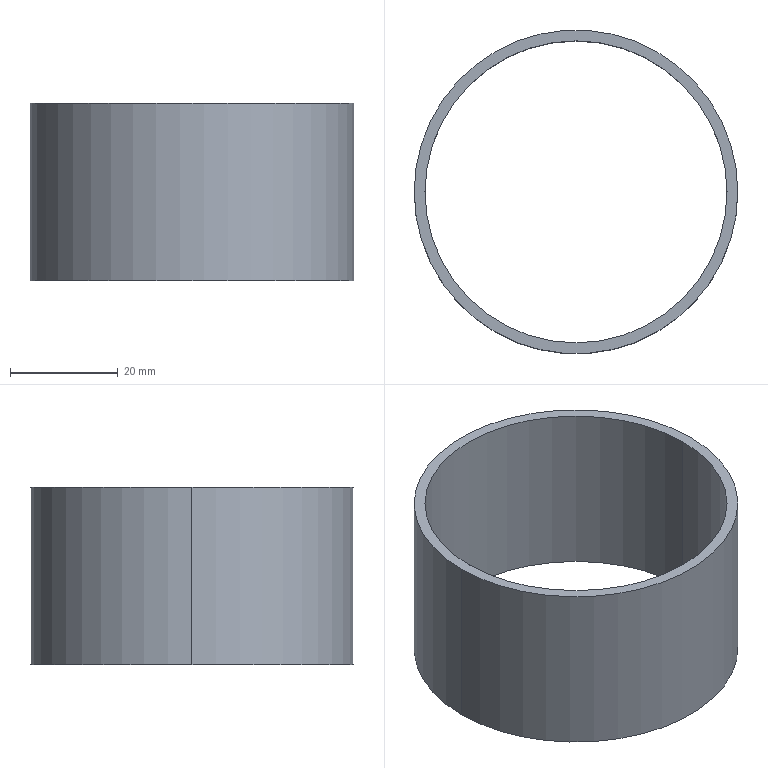Part | SolidWorks | features Extrusion 1 | 1 solid | 6 faces | box 60 x 60 x 33 mm | volume 12026 mm3 | cylinder 4 | plane 2 | commonest cylinder face diameters 56 x2 60 x2
STEP:
#1=CARTESIAN_POINT('',(-28.,0.,33.));
#2=VERTEX_POINT('',#1);
#3=CARTESIAN_POINT('',(28.,0.,33.));
#4=VERTEX_POINT('',#3);
#5=CARTESIAN_POINT('',(0.,0.,33.));
#6=DIRECTION('',(0.,0.,1.));
#7=DIRECTION('',(1.,0.,0.));
#8=AXIS2_PLACEMENT_3D('',#5,#6,#7);
#9=CIRCLE('',#8,28.);
#10=EDGE_CURVE('',#2,#4,#9,.T.);
#11=ORIENTED_EDGE('',*,*,#10,.T.);
#12=CARTESIAN_POINT('',(28.,0.,0.));
#13=VERTEX_POINT('',#12);
#14=CARTESIAN_POINT('',(28.,0.,33.));
#15=DIRECTION('',(0.,0.,-1.));
#16=VECTOR('',#15,1000.);
#17=LINE('',#14,#16);
#18=EDGE_CURVE('',#4,#13,#17,.T.);
#19=ORIENTED_EDGE('',*,*,#18,.T.);
#20=CARTESIAN_POINT('',(-28.,0.,0.));
#21=VERTEX_POINT('',#20);
#22=CARTESIAN_POINT('',(0.,0.,0.));
#23=DIRECTION('',(0.,0.,1.));
#24=DIRECTION('',(1.,0.,0.));
#25=AXIS2_PLACEMENT_3D('',#22,#23,#24);
#26=CIRCLE('',#25,28.);
#27=EDGE_CURVE('',#21,#13,#26,.T.);
#28=ORIENTED_EDGE('',*,*,#27,.F.);
#29=CARTESIAN_POINT('',(-28.,0.,33.));
#30=DIRECTION('',(0.,0.,-1.));
#31=VECTOR('',#30,1000.);
#32=LINE('',#29,#31);
#33=EDGE_CURVE('',#2,#21,#32,.T.);
#34=ORIENTED_EDGE('',*,*,#33,.F.);
#35=EDGE_LOOP('',(#11,#19,#28,#34));
#36=FACE_OUTER_BOUND('',#35,.T.);
#37=CARTESIAN_POINT('',(0.,0.,33.));
#38=DIRECTION('',(0.,0.,-1.));
#39=DIRECTION('',(-1.,0.,0.));
#40=AXIS2_PLACEMENT_3D('',#37,#38,#39);
#41=CYLINDRICAL_SURFACE('',#40,28.);
#42=ADVANCED_FACE('',(#36),#41,.F.);
#43=CARTESIAN_POINT('',(30.,0.,33.));
#44=VERTEX_POINT('',#43);
#45=CARTESIAN_POINT('',(-30.,0.,33.));
#46=VERTEX_POINT('',#45);
#47=CARTESIAN_POINT('',(0.,0.,33.));
#48=DIRECTION('',(0.,0.,1.));
#49=DIRECTION('',(1.,0.,0.));
#50=AXIS2_PLACEMENT_3D('',#47,#48,#49);
#51=CIRCLE('',#50,30.);
#52=EDGE_CURVE('',#44,#46,#51,.T.);
#53=ORIENTED_EDGE('',*,*,#52,.F.);
#54=CARTESIAN_POINT('',(30.,0.,0.));
#55=VERTEX_POINT('',#54);
#56=CARTESIAN_POINT('',(30.,0.,33.));
#57=DIRECTION('',(0.,0.,-1.));
#58=VECTOR('',#57,1000.);
#59=LINE('',#56,#58);
#60=EDGE_CURVE('',#44,#55,#59,.T.);
#61=ORIENTED_EDGE('',*,*,#60,.T.);
#62=CARTESIAN_POINT('',(-30.,0.,0.));
#63=VERTEX_POINT('',#62);
#64=CARTESIAN_POINT('',(0.,0.,0.));
#65=DIRECTION('',(0.,0.,1.));
#66=DIRECTION('',(1.,0.,0.));
#67=AXIS2_PLACEMENT_3D('',#64,#65,#66);
#68=CIRCLE('',#67,30.);
#69=EDGE_CURVE('',#55,#63,#68,.T.);
#70=ORIENTED_EDGE('',*,*,#69,.T.);
#71=CARTESIAN_POINT('',(-30.,0.,33.));
#72=DIRECTION('',(0.,0.,-1.));
#73=VECTOR('',#72,1000.);
#74=LINE('',#71,#73);
#75=EDGE_CURVE('',#46,#63,#74,.T.);
#76=ORIENTED_EDGE('',*,*,#75,.F.);
#77=EDGE_LOOP('',(#53,#61,#70,#76));
#78=FACE_OUTER_BOUND('',#77,.T.);
#79=CARTESIAN_POINT('',(0.,0.,33.));
#80=DIRECTION('',(0.,0.,-1.));
#81=DIRECTION('',(-1.,0.,0.));
#82=AXIS2_PLACEMENT_3D('',#79,#80,#81);
#83=CYLINDRICAL_SURFACE('',#82,30.);
#84=ADVANCED_FACE('',(#78),#83,.T.);
#85=CARTESIAN_POINT('',(0.,0.,33.));
#86=DIRECTION('',(0.,0.,1.));
#87=DIRECTION('',(1.,0.,0.));
#88=AXIS2_PLACEMENT_3D('',#85,#86,#87);
#89=CIRCLE('',#88,30.);
#90=EDGE_CURVE('',#46,#44,#89,.T.);
#91=ORIENTED_EDGE('',*,*,#90,.T.);
#92=ORIENTED_EDGE('',*,*,#52,.T.);
#93=EDGE_LOOP('',(#91,#92));
#94=FACE_OUTER_BOUND('',#93,.T.);
#95=ORIENTED_EDGE('',*,*,#10,.F.);
#96=CARTESIAN_POINT('',(0.,0.,33.));
#97=DIRECTION('',(0.,0.,1.));
#98=DIRECTION('',(1.,0.,0.));
#99=AXIS2_PLACEMENT_3D('',#96,#97,#98);
#100=CIRCLE('',#99,28.);
#101=EDGE_CURVE('',#4,#2,#100,.T.);
#102=ORIENTED_EDGE('',*,*,#101,.F.);
#103=EDGE_LOOP('',(#95,#102));
#104=FACE_BOUND('',#103,.T.);
#105=CARTESIAN_POINT('',(0.,0.,33.));
#106=DIRECTION('',(0.,0.,1.));
#107=DIRECTION('',(1.,0.,0.));
#108=AXIS2_PLACEMENT_3D('',#105,#106,#107);
#109=PLANE('',#108);
#110=ADVANCED_FACE('',(#94,#104),#109,.T.);
#111=CARTESIAN_POINT('',(0.,0.,0.));
#112=DIRECTION('',(0.,0.,1.));
#113=DIRECTION('',(1.,0.,0.));
#114=AXIS2_PLACEMENT_3D('',#111,#112,#113);
#115=CIRCLE('',#114,30.);
#116=EDGE_CURVE('',#63,#55,#115,.T.);
#117=ORIENTED_EDGE('',*,*,#116,.F.);
#118=ORIENTED_EDGE('',*,*,#69,.F.);
#119=EDGE_LOOP('',(#117,#118));
#120=FACE_OUTER_BOUND('',#119,.T.);
#121=ORIENTED_EDGE('',*,*,#27,.T.);
#122=CARTESIAN_POINT('',(0.,0.,0.));
#123=DIRECTION('',(0.,0.,1.));
#124=DIRECTION('',(1.,0.,0.));
#125=AXIS2_PLACEMENT_3D('',#122,#123,#124);
#126=CIRCLE('',#125,28.);
#127=EDGE_CURVE('',#13,#21,#126,.T.);
#128=ORIENTED_EDGE('',*,*,#127,.T.);
#129=EDGE_LOOP('',(#121,#128));
#130=FACE_BOUND('',#129,.T.);
#131=CARTESIAN_POINT('',(0.,0.,0.));
#132=DIRECTION('',(0.,0.,1.));
#133=DIRECTION('',(1.,0.,0.));
#134=AXIS2_PLACEMENT_3D('',#131,#132,#133);
#135=PLANE('',#134);
#136=ADVANCED_FACE('',(#120,#130),#135,.F.);
#137=ORIENTED_EDGE('',*,*,#60,.F.);
#138=ORIENTED_EDGE('',*,*,#90,.F.);
#139=ORIENTED_EDGE('',*,*,#75,.T.);
#140=ORIENTED_EDGE('',*,*,#116,.T.);
#141=EDGE_LOOP('',(#137,#138,#139,#140));
#142=FACE_OUTER_BOUND('',#141,.T.);
#143=CARTESIAN_POINT('',(0.,0.,33.));
#144=DIRECTION('',(0.,0.,-1.));
#145=DIRECTION('',(-1.,0.,0.));
#146=AXIS2_PLACEMENT_3D('',#143,#144,#145);
#147=CYLINDRICAL_SURFACE('',#146,30.);
#148=ADVANCED_FACE('',(#142),#147,.T.);
#149=ORIENTED_EDGE('',*,*,#18,.F.);
#150=ORIENTED_EDGE('',*,*,#101,.T.);
#151=ORIENTED_EDGE('',*,*,#33,.T.);
#152=ORIENTED_EDGE('',*,*,#127,.F.);
#153=EDGE_LOOP('',(#149,#150,#151,#152));
#154=FACE_OUTER_BOUND('',#153,.T.);
#155=CARTESIAN_POINT('',(0.,0.,33.));
#156=DIRECTION('',(0.,0.,-1.));
#157=DIRECTION('',(-1.,0.,0.));
#158=AXIS2_PLACEMENT_3D('',#155,#156,#157);
#159=CYLINDRICAL_SURFACE('',#158,28.);
#160=ADVANCED_FACE('',(#154),#159,.F.);
#161=CLOSED_SHELL('',(#42,#84,#110,#136,#148,#160));
#162=MANIFOLD_SOLID_BREP('',#161);
#163=CARTESIAN_POINT('',(0.,0.,0.));
#164=DIRECTION('',(0.,0.,1.));
#165=DIRECTION('',(1.,0.,0.));
#166=AXIS2_PLACEMENT_3D('',#163,#164,#165);
#167=(LENGTH_UNIT()NAMED_UNIT(*)SI_UNIT(.MILLI.,.METRE.));
#168=UNCERTAINTY_MEASURE_WITH_UNIT(LENGTH_MEASURE(0.00001),#167,'','');
#169=(NAMED_UNIT(*)PLANE_ANGLE_UNIT()SI_UNIT($,.RADIAN.));
#170=(NAMED_UNIT(*)SI_UNIT($,.STERADIAN.)SOLID_ANGLE_UNIT());
#171=(GEOMETRIC_REPRESENTATION_CONTEXT(3)GLOBAL_UNCERTAINTY_ASSIGNED_CONTEXT((#168))GLOBAL_UNIT_ASSIGNED_CONTEXT((#167,#169,#170))REPRESENTATION_CONTEXT('',''));
#172=ADVANCED_BREP_SHAPE_REPRESENTATION('',(#162,#166),#171);